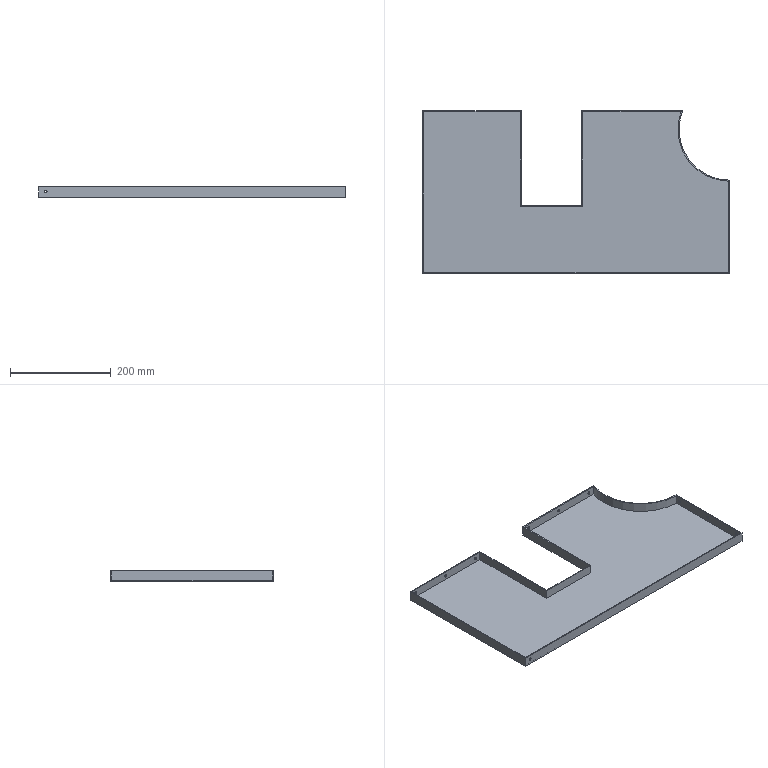Part | SolidWorks | features ICE 3, Extrusion 1, Shell 1 | 1 solid | 43 faces | box 609 x 323 x 20 mm | volume 403774 mm3 | cylinder 24 | plane 19 | commonest cylinder face diameters 5.5 x20 200 x2 204 x2
STEP:
#1=CARTESIAN_POINT('',(609.,174.,8.25));
#2=VERTEX_POINT('',#1);
#3=CARTESIAN_POINT('',(609.,174.,13.75));
#4=VERTEX_POINT('',#3);
#5=CARTESIAN_POINT('',(609.,174.,11.));
#6=DIRECTION('',(-1.,0.,0.));
#7=DIRECTION('',(0.,0.,1.));
#8=AXIS2_PLACEMENT_3D('',#5,#6,#7);
#9=CIRCLE('',#8,2.75);
#10=EDGE_CURVE('',#2,#4,#9,.T.);
#11=ORIENTED_EDGE('',*,*,#10,.F.);
#12=CARTESIAN_POINT('',(607.,174.,8.25));
#13=VERTEX_POINT('',#12);
#14=CARTESIAN_POINT('',(617.,174.,8.25));
#15=DIRECTION('',(-1.,0.,0.));
#16=VECTOR('',#15,1000.);
#17=LINE('',#14,#16);
#18=EDGE_CURVE('',#2,#13,#17,.T.);
#19=ORIENTED_EDGE('',*,*,#18,.T.);
#20=CARTESIAN_POINT('',(607.,174.,13.75));
#21=VERTEX_POINT('',#20);
#22=CARTESIAN_POINT('',(607.,174.,11.));
#23=DIRECTION('',(-1.,0.,0.));
#24=DIRECTION('',(0.,0.,1.));
#25=AXIS2_PLACEMENT_3D('',#22,#23,#24);
#26=CIRCLE('',#25,2.75);
#27=EDGE_CURVE('',#13,#21,#26,.T.);
#28=ORIENTED_EDGE('',*,*,#27,.T.);
#29=CARTESIAN_POINT('',(617.,174.,13.75));
#30=DIRECTION('',(-1.,0.,0.));
#31=VECTOR('',#30,1000.);
#32=LINE('',#29,#31);
#33=EDGE_CURVE('',#4,#21,#32,.T.);
#34=ORIENTED_EDGE('',*,*,#33,.F.);
#35=EDGE_LOOP('',(#11,#19,#28,#34));
#36=FACE_OUTER_BOUND('',#35,.T.);
#37=CARTESIAN_POINT('',(617.,174.,11.));
#38=DIRECTION('',(-1.,0.,0.));
#39=DIRECTION('',(0.,0.,1.));
#40=AXIS2_PLACEMENT_3D('',#37,#38,#39);
#41=CYLINDRICAL_SURFACE('',#40,2.75);
#42=ADVANCED_FACE('',(#36),#41,.F.);
#43=CARTESIAN_POINT('',(609.,94.,8.25));
#44=VERTEX_POINT('',#43);
#45=CARTESIAN_POINT('',(609.,94.,13.75));
#46=VERTEX_POINT('',#45);
#47=CARTESIAN_POINT('',(609.,94.,11.));
#48=DIRECTION('',(-1.,0.,0.));
#49=DIRECTION('',(0.,0.,1.));
#50=AXIS2_PLACEMENT_3D('',#47,#48,#49);
#51=CIRCLE('',#50,2.75);
#52=EDGE_CURVE('',#44,#46,#51,.T.);
#53=ORIENTED_EDGE('',*,*,#52,.F.);
#54=CARTESIAN_POINT('',(607.,94.,8.25));
#55=VERTEX_POINT('',#54);
#56=CARTESIAN_POINT('',(617.,94.,8.25));
#57=DIRECTION('',(-1.,0.,0.));
#58=VECTOR('',#57,1000.);
#59=LINE('',#56,#58);
#60=EDGE_CURVE('',#44,#55,#59,.T.);
#61=ORIENTED_EDGE('',*,*,#60,.T.);
#62=CARTESIAN_POINT('',(607.,94.,13.75));
#63=VERTEX_POINT('',#62);
#64=CARTESIAN_POINT('',(607.,94.,11.));
#65=DIRECTION('',(-1.,0.,0.));
#66=DIRECTION('',(0.,0.,1.));
#67=AXIS2_PLACEMENT_3D('',#64,#65,#66);
#68=CIRCLE('',#67,2.75);
#69=EDGE_CURVE('',#55,#63,#68,.T.);
#70=ORIENTED_EDGE('',*,*,#69,.T.);
#71=CARTESIAN_POINT('',(617.,94.,13.75));
#72=DIRECTION('',(-1.,0.,0.));
#73=VECTOR('',#72,1000.);
#74=LINE('',#71,#73);
#75=EDGE_CURVE('',#46,#63,#74,.T.);
#76=ORIENTED_EDGE('',*,*,#75,.F.);
#77=EDGE_LOOP('',(#53,#61,#70,#76));
#78=FACE_OUTER_BOUND('',#77,.T.);
#79=CARTESIAN_POINT('',(617.,94.,11.));
#80=DIRECTION('',(-1.,0.,0.));
#81=DIRECTION('',(0.,0.,1.));
#82=AXIS2_PLACEMENT_3D('',#79,#80,#81);
#83=CYLINDRICAL_SURFACE('',#82,2.75);
#84=ADVANCED_FACE('',(#78),#83,.F.);
#85=CARTESIAN_POINT('',(609.,14.,8.25));
#86=VERTEX_POINT('',#85);
#87=CARTESIAN_POINT('',(609.,14.,13.75));
#88=VERTEX_POINT('',#87);
#89=CARTESIAN_POINT('',(609.,14.,11.));
#90=DIRECTION('',(-1.,0.,0.));
#91=DIRECTION('',(0.,0.,1.));
#92=AXIS2_PLACEMENT_3D('',#89,#90,#91);
#93=CIRCLE('',#92,2.75);
#94=EDGE_CURVE('',#86,#88,#93,.T.);
#95=ORIENTED_EDGE('',*,*,#94,.F.);
#96=CARTESIAN_POINT('',(607.,14.,8.25));
#97=VERTEX_POINT('',#96);
#98=CARTESIAN_POINT('',(617.,14.,8.25));
#99=DIRECTION('',(-1.,0.,0.));
#100=VECTOR('',#99,1000.);
#101=LINE('',#98,#100);
#102=EDGE_CURVE('',#86,#97,#101,.T.);
#103=ORIENTED_EDGE('',*,*,#102,.T.);
#104=CARTESIAN_POINT('',(607.,14.,13.75));
#105=VERTEX_POINT('',#104);
#106=CARTESIAN_POINT('',(607.,14.,11.));
#107=DIRECTION('',(-1.,0.,0.));
#108=DIRECTION('',(0.,0.,1.));
#109=AXIS2_PLACEMENT_3D('',#106,#107,#108);
#110=CIRCLE('',#109,2.75);
#111=EDGE_CURVE('',#97,#105,#110,.T.);
#112=ORIENTED_EDGE('',*,*,#111,.T.);
#113=CARTESIAN_POINT('',(617.,14.,13.75));
#114=DIRECTION('',(-1.,0.,0.));
#115=VECTOR('',#114,1000.);
#116=LINE('',#113,#115);
#117=EDGE_CURVE('',#88,#105,#116,.T.);
#118=ORIENTED_EDGE('',*,*,#117,.F.);
#119=EDGE_LOOP('',(#95,#103,#112,#118));
#120=FACE_OUTER_BOUND('',#119,.T.);
#121=CARTESIAN_POINT('',(617.,14.,11.));
#122=DIRECTION('',(-1.,0.,0.));
#123=DIRECTION('',(0.,0.,1.));
#124=AXIS2_PLACEMENT_3D('',#121,#122,#123);
#125=CYLINDRICAL_SURFACE('',#124,2.75);
#126=ADVANCED_FACE('',(#120),#125,.F.);
#127=CARTESIAN_POINT('',(500.,323.,13.75));
#128=VERTEX_POINT('',#127);
#129=CARTESIAN_POINT('',(500.,323.,8.25));
#130=VERTEX_POINT('',#129);
#131=CARTESIAN_POINT('',(500.,323.,11.));
#132=DIRECTION('',(0.,-1.,0.));
#133=DIRECTION('',(1.,0.,0.));
#134=AXIS2_PLACEMENT_3D('',#131,#132,#133);
#135=CIRCLE('',#134,2.75);
#136=EDGE_CURVE('',#128,#130,#135,.T.);
#137=ORIENTED_EDGE('',*,*,#136,.F.);
#138=CARTESIAN_POINT('',(500.,321.,13.75));
#139=VERTEX_POINT('',#138);
#140=CARTESIAN_POINT('',(500.,331.,13.75));
#141=DIRECTION('',(0.,-1.,0.));
#142=VECTOR('',#141,1000.);
#143=LINE('',#140,#142);
#144=EDGE_CURVE('',#128,#139,#143,.T.);
#145=ORIENTED_EDGE('',*,*,#144,.T.);
#146=CARTESIAN_POINT('',(500.,321.,8.25));
#147=VERTEX_POINT('',#146);
#148=CARTESIAN_POINT('',(500.,321.,11.));
#149=DIRECTION('',(0.,-1.,0.));
#150=DIRECTION('',(0.,0.,-1.));
#151=AXIS2_PLACEMENT_3D('',#148,#149,#150);
#152=CIRCLE('',#151,2.75);
#153=EDGE_CURVE('',#139,#147,#152,.T.);
#154=ORIENTED_EDGE('',*,*,#153,.T.);
#155=CARTESIAN_POINT('',(500.,331.,8.25));
#156=DIRECTION('',(0.,-1.,0.));
#157=VECTOR('',#156,1000.);
#158=LINE('',#155,#157);
#159=EDGE_CURVE('',#130,#147,#158,.T.);
#160=ORIENTED_EDGE('',*,*,#159,.F.);
#161=EDGE_LOOP('',(#137,#145,#154,#160));
#162=FACE_OUTER_BOUND('',#161,.T.);
#163=CARTESIAN_POINT('',(500.,331.,11.));
#164=DIRECTION('',(0.,-1.,0.));
#165=DIRECTION('',(0.,0.,-1.));
#166=AXIS2_PLACEMENT_3D('',#163,#164,#165);
#167=CYLINDRICAL_SURFACE('',#166,2.75);
#168=ADVANCED_FACE('',(#162),#167,.F.);
#169=CARTESIAN_POINT('',(415.,323.,13.75));
#170=VERTEX_POINT('',#169);
#171=CARTESIAN_POINT('',(415.,323.,8.25));
#172=VERTEX_POINT('',#171);
#173=CARTESIAN_POINT('',(415.,323.,11.));
#174=DIRECTION('',(0.,-1.,0.));
#175=DIRECTION('',(1.,0.,0.));
#176=AXIS2_PLACEMENT_3D('',#173,#174,#175);
#177=CIRCLE('',#176,2.75);
#178=EDGE_CURVE('',#170,#172,#177,.T.);
#179=ORIENTED_EDGE('',*,*,#178,.F.);
#180=CARTESIAN_POINT('',(415.,321.,13.75));
#181=VERTEX_POINT('',#180);
#182=CARTESIAN_POINT('',(415.,331.,13.75));
#183=DIRECTION('',(0.,-1.,0.));
#184=VECTOR('',#183,1000.);
#185=LINE('',#182,#184);
#186=EDGE_CURVE('',#170,#181,#185,.T.);
#187=ORIENTED_EDGE('',*,*,#186,.T.);
#188=CARTESIAN_POINT('',(415.,321.,8.25));
#189=VERTEX_POINT('',#188);
#190=CARTESIAN_POINT('',(415.,321.,11.));
#191=DIRECTION('',(0.,-1.,0.));
#192=DIRECTION('',(0.,0.,-1.));
#193=AXIS2_PLACEMENT_3D('',#190,#191,#192);
#194=CIRCLE('',#193,2.75);
#195=EDGE_CURVE('',#181,#189,#194,.T.);
#196=ORIENTED_EDGE('',*,*,#195,.T.);
#197=CARTESIAN_POINT('',(415.,331.,8.25));
#198=DIRECTION('',(0.,-1.,0.));
#199=VECTOR('',#198,1000.);
#200=LINE('',#197,#199);
#201=EDGE_CURVE('',#172,#189,#200,.T.);
#202=ORIENTED_EDGE('',*,*,#201,.F.);
#203=EDGE_LOOP('',(#179,#187,#196,#202));
#204=FACE_OUTER_BOUND('',#203,.T.);
#205=CARTESIAN_POINT('',(415.,331.,11.));
#206=DIRECTION('',(0.,-1.,0.));
#207=DIRECTION('',(0.,0.,-1.));
#208=AXIS2_PLACEMENT_3D('',#205,#206,#207);
#209=CYLINDRICAL_SURFACE('',#208,2.75);
#210=ADVANCED_FACE('',(#204),#209,.F.);
#211=CARTESIAN_POINT('',(330.,323.,13.75));
#212=VERTEX_POINT('',#211);
#213=CARTESIAN_POINT('',(330.,323.,8.25));
#214=VERTEX_POINT('',#213);
#215=CARTESIAN_POINT('',(330.,323.,11.));
#216=DIRECTION('',(0.,-1.,0.));
#217=DIRECTION('',(1.,0.,0.));
#218=AXIS2_PLACEMENT_3D('',#215,#216,#217);
#219=CIRCLE('',#218,2.75);
#220=EDGE_CURVE('',#212,#214,#219,.T.);
#221=ORIENTED_EDGE('',*,*,#220,.F.);
#222=CARTESIAN_POINT('',(330.,321.,13.75));
#223=VERTEX_POINT('',#222);
#224=CARTESIAN_POINT('',(330.,331.,13.75));
#225=DIRECTION('',(0.,-1.,0.));
#226=VECTOR('',#225,1000.);
#227=LINE('',#224,#226);
#228=EDGE_CURVE('',#212,#223,#227,.T.);
#229=ORIENTED_EDGE('',*,*,#228,.T.);
#230=CARTESIAN_POINT('',(330.,321.,8.25));
#231=VERTEX_POINT('',#230);
#232=CARTESIAN_POINT('',(330.,321.,11.));
#233=DIRECTION('',(0.,-1.,0.));
#234=DIRECTION('',(0.,0.,-1.));
#235=AXIS2_PLACEMENT_3D('',#232,#233,#234);
#236=CIRCLE('',#235,2.75);
#237=EDGE_CURVE('',#223,#231,#236,.T.);
#238=ORIENTED_EDGE('',*,*,#237,.T.);
#239=CARTESIAN_POINT('',(330.,331.,8.25));
#240=DIRECTION('',(0.,-1.,0.));
#241=VECTOR('',#240,1000.);
#242=LINE('',#239,#241);
#243=EDGE_CURVE('',#214,#231,#242,.T.);
#244=ORIENTED_EDGE('',*,*,#243,.F.);
#245=EDGE_LOOP('',(#221,#229,#238,#244));
#246=FACE_OUTER_BOUND('',#245,.T.);
#247=CARTESIAN_POINT('',(330.,331.,11.));
#248=DIRECTION('',(0.,-1.,0.));
#249=DIRECTION('',(0.,0.,-1.));
#250=AXIS2_PLACEMENT_3D('',#247,#248,#249);
#251=CYLINDRICAL_SURFACE('',#250,2.75);
#252=ADVANCED_FACE('',(#246),#251,.F.);
#253=CARTESIAN_POINT('',(182.,323.,13.75));
#254=VERTEX_POINT('',#253);
#255=CARTESIAN_POINT('',(182.,323.,8.25));
#256=VERTEX_POINT('',#255);
#257=CARTESIAN_POINT('',(182.,323.,11.));
#258=DIRECTION('',(0.,-1.,0.));
#259=DIRECTION('',(0.,0.,-1.));
#260=AXIS2_PLACEMENT_3D('',#257,#258,#259);
#261=CIRCLE('',#260,2.75);
#262=EDGE_CURVE('',#254,#256,#261,.T.);
#263=ORIENTED_EDGE('',*,*,#262,.F.);
#264=CARTESIAN_POINT('',(182.,321.,13.75));
#265=VERTEX_POINT('',#264);
#266=CARTESIAN_POINT('',(182.,331.,13.75));
#267=DIRECTION('',(0.,-1.,0.));
#268=VECTOR('',#267,1000.);
#269=LINE('',#266,#268);
#270=EDGE_CURVE('',#254,#265,#269,.T.);
#271=ORIENTED_EDGE('',*,*,#270,.T.);
#272=CARTESIAN_POINT('',(182.,321.,8.25));
#273=VERTEX_POINT('',#272);
#274=CARTESIAN_POINT('',(182.,321.,11.));
#275=DIRECTION('',(0.,-1.,0.));
#276=DIRECTION('',(0.,0.,-1.));
#277=AXIS2_PLACEMENT_3D('',#274,#275,#276);
#278=CIRCLE('',#277,2.75);
#279=EDGE_CURVE('',#265,#273,#278,.T.);
#280=ORIENTED_EDGE('',*,*,#279,.T.);
#281=CARTESIAN_POINT('',(182.,331.,8.25));
#282=DIRECTION('',(0.,-1.,0.));
#283=VECTOR('',#282,1000.);
#284=LINE('',#281,#283);
#285=EDGE_CURVE('',#256,#273,#284,.T.);
#286=ORIENTED_EDGE('',*,*,#285,.F.);
#287=EDGE_LOOP('',(#263,#271,#280,#286));
#288=FACE_OUTER_BOUND('',#287,.T.);
#289=CARTESIAN_POINT('',(182.,331.,11.));
#290=DIRECTION('',(0.,-1.,0.));
#291=DIRECTION('',(0.,0.,-1.));
#292=AXIS2_PLACEMENT_3D('',#289,#290,#291);
#293=CYLINDRICAL_SURFACE('',#292,2.75);
#294=ADVANCED_FACE('',(#288),#293,.F.);
#295=CARTESIAN_POINT('',(98.,323.,13.75));
#296=VERTEX_POINT('',#295);
#297=CARTESIAN_POINT('',(98.,323.,8.25));
#298=VERTEX_POINT('',#297);
#299=CARTESIAN_POINT('',(98.,323.,11.));
#300=DIRECTION('',(0.,-1.,0.));
#301=DIRECTION('',(0.,0.,-1.));
#302=AXIS2_PLACEMENT_3D('',#299,#300,#301);
#303=CIRCLE('',#302,2.75);
#304=EDGE_CURVE('',#296,#298,#303,.T.);
#305=ORIENTED_EDGE('',*,*,#304,.F.);
#306=CARTESIAN_POINT('',(98.,321.,13.75));
#307=VERTEX_POINT('',#306);
#308=CARTESIAN_POINT('',(98.,331.,13.75));
#309=DIRECTION('',(0.,-1.,0.));
#310=VECTOR('',#309,1000.);
#311=LINE('',#308,#310);
#312=EDGE_CURVE('',#296,#307,#311,.T.);
#313=ORIENTED_EDGE('',*,*,#312,.T.);
#314=CARTESIAN_POINT('',(98.,321.,8.25));
#315=VERTEX_POINT('',#314);
#316=CARTESIAN_POINT('',(98.,321.,11.));
#317=DIRECTION('',(0.,-1.,0.));
#318=DIRECTION('',(0.,0.,-1.));
#319=AXIS2_PLACEMENT_3D('',#316,#317,#318);
#320=CIRCLE('',#319,2.75);
#321=EDGE_CURVE('',#307,#315,#320,.T.);
#322=ORIENTED_EDGE('',*,*,#321,.T.);
#323=CARTESIAN_POINT('',(98.,331.,8.25));
#324=DIRECTION('',(0.,-1.,0.));
#325=VECTOR('',#324,1000.);
#326=LINE('',#323,#325);
#327=EDGE_CURVE('',#298,#315,#326,.T.);
#328=ORIENTED_EDGE('',*,*,#327,.F.);
#329=EDGE_LOOP('',(#305,#313,#322,#328));
#330=FACE_OUTER_BOUND('',#329,.T.);
#331=CARTESIAN_POINT('',(98.,331.,11.));
#332=DIRECTION('',(0.,-1.,0.));
#333=DIRECTION('',(0.,0.,-1.));
#334=AXIS2_PLACEMENT_3D('',#331,#332,#333);
#335=CYLINDRICAL_SURFACE('',#334,2.75);
#336=ADVANCED_FACE('',(#330),#335,.F.);
#337=CARTESIAN_POINT('',(14.,2.,13.75));
#338=VERTEX_POINT('',#337);
#339=CARTESIAN_POINT('',(14.,2.,8.25));
#340=VERTEX_POINT('',#339);
#341=CARTESIAN_POINT('',(14.,2.,11.));
#342=DIRECTION('',(0.,-1.,0.));
#343=DIRECTION('',(0.,0.,1.));
#344=AXIS2_PLACEMENT_3D('',#341,#342,#343);
#345=CIRCLE('',#344,2.75);
#346=EDGE_CURVE('',#338,#340,#345,.T.);
#347=ORIENTED_EDGE('',*,*,#346,.F.);
#348=CARTESIAN_POINT('',(14.,0.,13.75));
#349=VERTEX_POINT('',#348);
#350=CARTESIAN_POINT('',(14.,340.,13.75));
#351=DIRECTION('',(0.,-1.,0.));
#352=VECTOR('',#351,1000.);
#353=LINE('',#350,#352);
#354=EDGE_CURVE('',#338,#349,#353,.T.);
#355=ORIENTED_EDGE('',*,*,#354,.T.);
#356=CARTESIAN_POINT('',(14.,0.,8.25));
#357=VERTEX_POINT('',#356);
#358=CARTESIAN_POINT('',(14.,0.,11.));
#359=DIRECTION('',(0.,-1.,0.));
#360=DIRECTION('',(0.,0.,1.));
#361=AXIS2_PLACEMENT_3D('',#358,#359,#360);
#362=CIRCLE('',#361,2.75);
#363=EDGE_CURVE('',#349,#357,#362,.T.);
#364=ORIENTED_EDGE('',*,*,#363,.T.);
#365=CARTESIAN_POINT('',(14.,340.,8.25));
#366=DIRECTION('',(0.,-1.,0.));
#367=VECTOR('',#366,1000.);
#368=LINE('',#365,#367);
#369=EDGE_CURVE('',#340,#357,#368,.T.);
#370=ORIENTED_EDGE('',*,*,#369,.F.);
#371=EDGE_LOOP('',(#347,#355,#364,#370));
#372=FACE_OUTER_BOUND('',#371,.T.);
#373=CARTESIAN_POINT('',(14.,340.,11.));
#374=DIRECTION('',(0.,-1.,0.));
#375=DIRECTION('',(0.,0.,-1.));
#376=AXIS2_PLACEMENT_3D('',#373,#374,#375);
#377=CYLINDRICAL_SURFACE('',#376,2.75);
#378=ADVANCED_FACE('',(#372),#377,.F.);
#379=CARTESIAN_POINT('',(14.,323.,8.25));
#380=VERTEX_POINT('',#379);
#381=CARTESIAN_POINT('',(14.,323.,13.75));
#382=VERTEX_POINT('',#381);
#383=CARTESIAN_POINT('',(14.,323.,11.));
#384=DIRECTION('',(0.,1.,0.));
#385=DIRECTION('',(0.,0.,-1.));
#386=AXIS2_PLACEMENT_3D('',#383,#384,#385);
#387=CIRCLE('',#386,2.75);
#388=EDGE_CURVE('',#380,#382,#387,.T.);
#389=ORIENTED_EDGE('',*,*,#388,.T.);
#390=CARTESIAN_POINT('',(14.,321.,13.75));
#391=VERTEX_POINT('',#390);
#392=CARTESIAN_POINT('',(14.,340.,13.75));
#393=DIRECTION('',(0.,-1.,0.));
#394=VECTOR('',#393,1000.);
#395=LINE('',#392,#394);
#396=EDGE_CURVE('',#382,#391,#395,.T.);
#397=ORIENTED_EDGE('',*,*,#396,.T.);
#398=CARTESIAN_POINT('',(14.,321.,8.25));
#399=VERTEX_POINT('',#398);
#400=CARTESIAN_POINT('',(14.,321.,11.));
#401=DIRECTION('',(0.,1.,0.));
#402=DIRECTION('',(0.,0.,-1.));
#403=AXIS2_PLACEMENT_3D('',#400,#401,#402);
#404=CIRCLE('',#403,2.75);
#405=EDGE_CURVE('',#399,#391,#404,.T.);
#406=ORIENTED_EDGE('',*,*,#405,.F.);
#407=CARTESIAN_POINT('',(14.,340.,8.25));
#408=DIRECTION('',(0.,-1.,0.));
#409=VECTOR('',#408,1000.);
#410=LINE('',#407,#409);
#411=EDGE_CURVE('',#380,#399,#410,.T.);
#412=ORIENTED_EDGE('',*,*,#411,.F.);
#413=EDGE_LOOP('',(#389,#397,#406,#412));
#414=FACE_OUTER_BOUND('',#413,.T.);
#415=CARTESIAN_POINT('',(14.,340.,11.));
#416=DIRECTION('',(0.,-1.,0.));
#417=DIRECTION('',(0.,0.,-1.));
#418=AXIS2_PLACEMENT_3D('',#415,#416,#417);
#419=CYLINDRICAL_SURFACE('',#418,2.75);
#420=ADVANCED_FACE('',(#414),#419,.F.);
#421=CARTESIAN_POINT('',(607.,183.02,20.));
#422=VERTEX_POINT('',#421);
#423=CARTESIAN_POINT('',(507.,285.,20.));
#424=VERTEX_POINT('',#423);
#425=CARTESIAN_POINT('',(609.,285.,20.));
#426=DIRECTION('',(0.,0.,-1.));
#427=DIRECTION('',(1.,0.,0.));
#428=AXIS2_PLACEMENT_3D('',#425,#426,#427);
#429=CIRCLE('',#428,102.);
#430=EDGE_CURVE('',#422,#424,#429,.T.);
#431=ORIENTED_EDGE('',*,*,#430,.T.);
#432=CARTESIAN_POINT('',(507.,285.,2.));
#433=VERTEX_POINT('',#432);
#434=CARTESIAN_POINT('',(507.,285.,20.));
#435=DIRECTION('',(0.,0.,-1.));
#436=VECTOR('',#435,1000.);
#437=LINE('',#434,#436);
#438=EDGE_CURVE('',#424,#433,#437,.T.);
#439=ORIENTED_EDGE('',*,*,#438,.T.);
#440=CARTESIAN_POINT('',(607.,183.02,2.));
#441=VERTEX_POINT('',#440);
#442=CARTESIAN_POINT('',(609.,285.,2.));
#443=DIRECTION('',(0.,0.,-1.));
#444=DIRECTION('',(1.,0.,0.));
#445=AXIS2_PLACEMENT_3D('',#442,#443,#444);
#446=CIRCLE('',#445,102.);
#447=EDGE_CURVE('',#441,#433,#446,.T.);
#448=ORIENTED_EDGE('',*,*,#447,.F.);
#449=CARTESIAN_POINT('',(607.,183.02,20.));
#450=DIRECTION('',(0.,0.,-1.));
#451=VECTOR('',#450,1000.);
#452=LINE('',#449,#451);
#453=EDGE_CURVE('',#422,#441,#452,.T.);
#454=ORIENTED_EDGE('',*,*,#453,.F.);
#455=EDGE_LOOP('',(#431,#439,#448,#454));
#456=FACE_OUTER_BOUND('',#455,.T.);
#457=CARTESIAN_POINT('',(609.,285.,20.));
#458=DIRECTION('',(0.,0.,-1.));
#459=DIRECTION('',(-1.,0.,0.));
#460=AXIS2_PLACEMENT_3D('',#457,#458,#459);
#461=CYLINDRICAL_SURFACE('',#460,102.);
#462=ADVANCED_FACE('',(#456),#461,.T.);
#463=CARTESIAN_POINT('',(509.,285.,20.));
#464=VERTEX_POINT('',#463);
#465=CARTESIAN_POINT('',(516.501,323.,20.));
#466=VERTEX_POINT('',#465);
#467=CARTESIAN_POINT('',(609.,285.,20.));
#468=DIRECTION('',(0.,0.,-1.));
#469=DIRECTION('',(1.,0.,0.));
#470=AXIS2_PLACEMENT_3D('',#467,#468,#469);
#471=CIRCLE('',#470,100.);
#472=EDGE_CURVE('',#464,#466,#471,.T.);
#473=ORIENTED_EDGE('',*,*,#472,.F.);
#474=CARTESIAN_POINT('',(509.,285.,0.));
#475=VERTEX_POINT('',#474);
#476=CARTESIAN_POINT('',(509.,285.,20.));
#477=DIRECTION('',(0.,0.,-1.));
#478=VECTOR('',#477,1000.);
#479=LINE('',#476,#478);
#480=EDGE_CURVE('',#464,#475,#479,.T.);
#481=ORIENTED_EDGE('',*,*,#480,.T.);
#482=CARTESIAN_POINT('',(516.501,323.,0.));
#483=VERTEX_POINT('',#482);
#484=CARTESIAN_POINT('',(609.,285.,0.));
#485=DIRECTION('',(0.,0.,-1.));
#486=DIRECTION('',(1.,0.,0.));
#487=AXIS2_PLACEMENT_3D('',#484,#485,#486);
#488=CIRCLE('',#487,100.);
#489=EDGE_CURVE('',#475,#483,#488,.T.);
#490=ORIENTED_EDGE('',*,*,#489,.T.);
#491=CARTESIAN_POINT('',(516.501,323.,20.));
#492=DIRECTION('',(0.,0.,-1.));
#493=VECTOR('',#492,1000.);
#494=LINE('',#491,#493);
#495=EDGE_CURVE('',#466,#483,#494,.T.);
#496=ORIENTED_EDGE('',*,*,#495,.F.);
#497=EDGE_LOOP('',(#473,#481,#490,#496));
#498=FACE_OUTER_BOUND('',#497,.T.);
#499=CARTESIAN_POINT('',(609.,285.,20.));
#500=DIRECTION('',(0.,0.,-1.));
#501=DIRECTION('',(-1.,0.,0.));
#502=AXIS2_PLACEMENT_3D('',#499,#500,#501);
#503=CYLINDRICAL_SURFACE('',#502,100.);
#504=ADVANCED_FACE('',(#498),#503,.F.);
#505=CARTESIAN_POINT('',(0.,0.,0.));
#506=VERTEX_POINT('',#505);
#507=CARTESIAN_POINT('',(609.,0.,0.));
#508=VERTEX_POINT('',#507);
#509=CARTESIAN_POINT('',(0.,0.,0.));
#510=DIRECTION('',(1.,0.,0.));
#511=VECTOR('',#510,1000.);
#512=LINE('',#509,#511);
#513=EDGE_CURVE('',#506,#508,#512,.T.);
#514=ORIENTED_EDGE('',*,*,#513,.T.);
#515=CARTESIAN_POINT('',(609.,0.,20.));
#516=VERTEX_POINT('',#515);
#517=CARTESIAN_POINT('',(609.,0.,20.));
#518=DIRECTION('',(0.,0.,-1.));
#519=VECTOR('',#518,1000.);
#520=LINE('',#517,#519);
#521=EDGE_CURVE('',#516,#508,#520,.T.);
#522=ORIENTED_EDGE('',*,*,#521,.F.);
#523=CARTESIAN_POINT('',(0.,0.,20.));
#524=VERTEX_POINT('',#523);
#525=CARTESIAN_POINT('',(0.,0.,20.));
#526=DIRECTION('',(1.,0.,0.));
#527=VECTOR('',#526,1000.);
#528=LINE('',#525,#527);
#529=EDGE_CURVE('',#524,#516,#528,.T.);
#530=ORIENTED_EDGE('',*,*,#529,.F.);
#531=CARTESIAN_POINT('',(0.,0.,20.));
#532=DIRECTION('',(0.,0.,-1.));
#533=VECTOR('',#532,1000.);
#534=LINE('',#531,#533);
#535=EDGE_CURVE('',#524,#506,#534,.T.);
#536=ORIENTED_EDGE('',*,*,#535,.T.);
#537=EDGE_LOOP('',(#514,#522,#530,#536));
#538=FACE_OUTER_BOUND('',#537,.T.);
#539=CARTESIAN_POINT('',(14.,0.,11.));
#540=DIRECTION('',(0.,-1.,0.));
#541=DIRECTION('',(0.,0.,1.));
#542=AXIS2_PLACEMENT_3D('',#539,#540,#541);
#543=CIRCLE('',#542,2.75);
#544=EDGE_CURVE('',#357,#349,#543,.T.);
#545=ORIENTED_EDGE('',*,*,#544,.F.);
#546=ORIENTED_EDGE('',*,*,#363,.F.);
#547=EDGE_LOOP('',(#545,#546));
#548=FACE_BOUND('',#547,.T.);
#549=CARTESIAN_POINT('',(0.,0.,20.));
#550=DIRECTION('',(0.,1.,0.));
#551=DIRECTION('',(0.,0.,1.));
#552=AXIS2_PLACEMENT_3D('',#549,#550,#551);
#553=PLANE('',#552);
#554=ADVANCED_FACE('',(#538,#548),#553,.F.);
#555=CARTESIAN_POINT('',(182.,323.,11.));
#556=DIRECTION('',(0.,-1.,0.));
#557=DIRECTION('',(0.,0.,-1.));
#558=AXIS2_PLACEMENT_3D('',#555,#556,#557);
#559=CIRCLE('',#558,2.75);
#560=EDGE_CURVE('',#256,#254,#559,.T.);
#561=ORIENTED_EDGE('',*,*,#560,.T.);
#562=ORIENTED_EDGE('',*,*,#262,.T.);
#563=EDGE_LOOP('',(#561,#562));
#564=FACE_BOUND('',#563,.T.);
#565=CARTESIAN_POINT('',(98.,323.,11.));
#566=DIRECTION('',(0.,-1.,0.));
#567=DIRECTION('',(0.,0.,-1.));
#568=AXIS2_PLACEMENT_3D('',#565,#566,#567);
#569=CIRCLE('',#568,2.75);
#570=EDGE_CURVE('',#298,#296,#569,.T.);
#571=ORIENTED_EDGE('',*,*,#570,.T.);
#572=ORIENTED_EDGE('',*,*,#304,.T.);
#573=EDGE_LOOP('',(#571,#572));
#574=FACE_BOUND('',#573,.T.);
#575=CARTESIAN_POINT('',(196.,323.,0.));
#576=VERTEX_POINT('',#575);
#577=CARTESIAN_POINT('',(0.,323.,0.));
#578=VERTEX_POINT('',#577);
#579=CARTESIAN_POINT('',(0.,323.,0.));
#580=DIRECTION('',(-1.,0.,0.));
#581=VECTOR('',#580,1000.);
#582=LINE('',#579,#581);
#583=EDGE_CURVE('',#576,#578,#582,.T.);
#584=ORIENTED_EDGE('',*,*,#583,.T.);
#585=CARTESIAN_POINT('',(0.,323.,20.));
#586=VERTEX_POINT('',#585);
#587=CARTESIAN_POINT('',(0.,323.,20.));
#588=DIRECTION('',(0.,0.,-1.));
#589=VECTOR('',#588,1000.);
#590=LINE('',#587,#589);
#591=EDGE_CURVE('',#586,#578,#590,.T.);
#592=ORIENTED_EDGE('',*,*,#591,.F.);
#593=CARTESIAN_POINT('',(196.,323.,20.));
#594=VERTEX_POINT('',#593);
#595=CARTESIAN_POINT('',(0.,323.,20.));
#596=DIRECTION('',(-1.,0.,0.));
#597=VECTOR('',#596,1000.);
#598=LINE('',#595,#597);
#599=EDGE_CURVE('',#594,#586,#598,.T.);
#600=ORIENTED_EDGE('',*,*,#599,.F.);
#601=CARTESIAN_POINT('',(196.,323.,20.));
#602=DIRECTION('',(0.,0.,-1.));
#603=VECTOR('',#602,1000.);
#604=LINE('',#601,#603);
#605=EDGE_CURVE('',#594,#576,#604,.T.);
#606=ORIENTED_EDGE('',*,*,#605,.T.);
#607=EDGE_LOOP('',(#584,#592,#600,#606));
#608=FACE_OUTER_BOUND('',#607,.T.);
#609=ORIENTED_EDGE('',*,*,#388,.F.);
#610=CARTESIAN_POINT('',(14.,323.,11.));
#611=DIRECTION('',(0.,1.,0.));
#612=DIRECTION('',(0.,0.,-1.));
#613=AXIS2_PLACEMENT_3D('',#610,#611,#612);
#614=CIRCLE('',#613,2.75);
#615=EDGE_CURVE('',#382,#380,#614,.T.);
#616=ORIENTED_EDGE('',*,*,#615,.F.);
#617=EDGE_LOOP('',(#609,#616));
#618=FACE_BOUND('',#617,.T.);
#619=CARTESIAN_POINT('',(0.,323.,20.));
#620=DIRECTION('',(0.,-1.,0.));
#621=DIRECTION('',(0.,0.,-1.));
#622=AXIS2_PLACEMENT_3D('',#619,#620,#621);
#623=PLANE('',#622);
#624=ADVANCED_FACE('',(#564,#574,#608,#618),#623,.F.);
#625=CARTESIAN_POINT('',(2.,2.,2.));
#626=VERTEX_POINT('',#625);
#627=CARTESIAN_POINT('',(607.,2.,2.));
#628=VERTEX_POINT('',#627);
#629=CARTESIAN_POINT('',(0.,2.,2.));
#630=DIRECTION('',(1.,0.,0.));
#631=VECTOR('',#630,1000.);
#632=LINE('',#629,#631);
#633=EDGE_CURVE('',#626,#628,#632,.T.);
#634=ORIENTED_EDGE('',*,*,#633,.F.);
#635=CARTESIAN_POINT('',(2.,2.,20.));
#636=VERTEX_POINT('',#635);
#637=CARTESIAN_POINT('',(2.,2.,20.));
#638=DIRECTION('',(0.,0.,-1.));
#639=VECTOR('',#638,1000.);
#640=LINE('',#637,#639);
#641=EDGE_CURVE('',#636,#626,#640,.T.);
#642=ORIENTED_EDGE('',*,*,#641,.F.);
#643=CARTESIAN_POINT('',(607.,2.,20.));
#644=VERTEX_POINT('',#643);
#645=CARTESIAN_POINT('',(0.,2.,20.));
#646=DIRECTION('',(1.,0.,0.));
#647=VECTOR('',#646,1000.);
#648=LINE('',#645,#647);
#649=EDGE_CURVE('',#636,#644,#648,.T.);
#650=ORIENTED_EDGE('',*,*,#649,.T.);
#651=CARTESIAN_POINT('',(607.,2.,20.));
#652=DIRECTION('',(0.,0.,-1.));
#653=VECTOR('',#652,1000.);
#654=LINE('',#651,#653);
#655=EDGE_CURVE('',#644,#628,#654,.T.);
#656=ORIENTED_EDGE('',*,*,#655,.T.);
#657=EDGE_LOOP('',(#634,#642,#650,#656));
#658=FACE_OUTER_BOUND('',#657,.T.);
#659=CARTESIAN_POINT('',(14.,2.,11.));
#660=DIRECTION('',(0.,-1.,0.));
#661=DIRECTION('',(0.,0.,1.));
#662=AXIS2_PLACEMENT_3D('',#659,#660,#661);
#663=CIRCLE('',#662,2.75);
#664=EDGE_CURVE('',#340,#338,#663,.T.);
#665=ORIENTED_EDGE('',*,*,#664,.T.);
#666=ORIENTED_EDGE('',*,*,#346,.T.);
#667=EDGE_LOOP('',(#665,#666));
#668=FACE_BOUND('',#667,.T.);
#669=CARTESIAN_POINT('',(0.,2.,20.));
#670=DIRECTION('',(0.,1.,0.));
#671=DIRECTION('',(0.,0.,1.));
#672=AXIS2_PLACEMENT_3D('',#669,#670,#671);
#673=PLANE('',#672);
#674=ADVANCED_FACE('',(#658,#668),#673,.T.);
#675=CARTESIAN_POINT('',(182.,321.,11.));
#676=DIRECTION('',(0.,-1.,0.));
#677=DIRECTION('',(0.,0.,-1.));
#678=AXIS2_PLACEMENT_3D('',#675,#676,#677);
#679=CIRCLE('',#678,2.75);
#680=EDGE_CURVE('',#273,#265,#679,.T.);
#681=ORIENTED_EDGE('',*,*,#680,.F.);
#682=ORIENTED_EDGE('',*,*,#279,.F.);
#683=EDGE_LOOP('',(#681,#682));
#684=FACE_BOUND('',#683,.T.);
#685=CARTESIAN_POINT('',(98.,321.,11.));
#686=DIRECTION('',(0.,-1.,0.));
#687=DIRECTION('',(0.,0.,-1.));
#688=AXIS2_PLACEMENT_3D('',#685,#686,#687);
#689=CIRCLE('',#688,2.75);
#690=EDGE_CURVE('',#315,#307,#689,.T.);
#691=ORIENTED_EDGE('',*,*,#690,.F.);
#692=ORIENTED_EDGE('',*,*,#321,.F.);
#693=EDGE_LOOP('',(#691,#692));
#694=FACE_BOUND('',#693,.T.);
#695=CARTESIAN_POINT('',(194.,321.,2.));
#696=VERTEX_POINT('',#695);
#697=CARTESIAN_POINT('',(2.,321.,2.));
#698=VERTEX_POINT('',#697);
#699=CARTESIAN_POINT('',(0.,321.,2.));
#700=DIRECTION('',(-1.,0.,0.));
#701=VECTOR('',#700,1000.);
#702=LINE('',#699,#701);
#703=EDGE_CURVE('',#696,#698,#702,.T.);
#704=ORIENTED_EDGE('',*,*,#703,.F.);
#705=CARTESIAN_POINT('',(194.,321.,20.));
#706=VERTEX_POINT('',#705);
#707=CARTESIAN_POINT('',(194.,321.,20.));
#708=DIRECTION('',(0.,0.,-1.));
#709=VECTOR('',#708,1000.);
#710=LINE('',#707,#709);
#711=EDGE_CURVE('',#706,#696,#710,.T.);
#712=ORIENTED_EDGE('',*,*,#711,.F.);
#713=CARTESIAN_POINT('',(2.,321.,20.));
#714=VERTEX_POINT('',#713);
#715=CARTESIAN_POINT('',(0.,321.,20.));
#716=DIRECTION('',(-1.,0.,0.));
#717=VECTOR('',#716,1000.);
#718=LINE('',#715,#717);
#719=EDGE_CURVE('',#706,#714,#718,.T.);
#720=ORIENTED_EDGE('',*,*,#719,.T.);
#721=CARTESIAN_POINT('',(2.,321.,20.));
#722=DIRECTION('',(0.,0.,-1.));
#723=VECTOR('',#722,1000.);
#724=LINE('',#721,#723);
#725=EDGE_CURVE('',#714,#698,#724,.T.);
#726=ORIENTED_EDGE('',*,*,#725,.T.);
#727=EDGE_LOOP('',(#704,#712,#720,#726));
#728=FACE_OUTER_BOUND('',#727,.T.);
#729=ORIENTED_EDGE('',*,*,#405,.T.);
#730=CARTESIAN_POINT('',(14.,321.,11.));
#731=DIRECTION('',(0.,1.,0.));
#732=DIRECTION('',(0.,0.,-1.));
#733=AXIS2_PLACEMENT_3D('',#730,#731,#732);
#734=CIRCLE('',#733,2.75);
#735=EDGE_CURVE('',#391,#399,#734,.T.);
#736=ORIENTED_EDGE('',*,*,#735,.T.);
#737=EDGE_LOOP('',(#729,#736));
#738=FACE_BOUND('',#737,.T.);
#739=CARTESIAN_POINT('',(0.,321.,20.));
#740=DIRECTION('',(0.,-1.,0.));
#741=DIRECTION('',(0.,0.,-1.));
#742=AXIS2_PLACEMENT_3D('',#739,#740,#741);
#743=PLANE('',#742);
#744=ADVANCED_FACE('',(#684,#694,#728,#738),#743,.T.);
#745=CARTESIAN_POINT('',(0.,0.,0.));
#746=DIRECTION('',(0.,-1.,0.));
#747=VECTOR('',#746,1000.);
#748=LINE('',#745,#747);
#749=EDGE_CURVE('',#578,#506,#748,.T.);
#750=ORIENTED_EDGE('',*,*,#749,.T.);
#751=ORIENTED_EDGE('',*,*,#535,.F.);
#752=CARTESIAN_POINT('',(0.,0.,20.));
#753=DIRECTION('',(0.,-1.,0.));
#754=VECTOR('',#753,1000.);
#755=LINE('',#752,#754);
#756=EDGE_CURVE('',#586,#524,#755,.T.);
#757=ORIENTED_EDGE('',*,*,#756,.F.);
#758=ORIENTED_EDGE('',*,*,#591,.T.);
#759=EDGE_LOOP('',(#750,#751,#757,#758));
#760=FACE_OUTER_BOUND('',#759,.T.);
#761=CARTESIAN_POINT('',(0.,0.,20.));
#762=DIRECTION('',(1.,0.,0.));
#763=DIRECTION('',(0.,0.,-1.));
#764=AXIS2_PLACEMENT_3D('',#761,#762,#763);
#765=PLANE('',#764);
#766=ADVANCED_FACE('',(#760),#765,.F.);
#767=CARTESIAN_POINT('',(609.,174.,11.));
#768=DIRECTION('',(-1.,0.,0.));
#769=DIRECTION('',(0.,0.,1.));
#770=AXIS2_PLACEMENT_3D('',#767,#768,#769);
#771=CIRCLE('',#770,2.75);
#772=EDGE_CURVE('',#4,#2,#771,.T.);
#773=ORIENTED_EDGE('',*,*,#772,.T.);
#774=ORIENTED_EDGE('',*,*,#10,.T.);
#775=EDGE_LOOP('',(#773,#774));
#776=FACE_BOUND('',#775,.T.);
#777=CARTESIAN_POINT('',(609.,94.,11.));
#778=DIRECTION('',(-1.,0.,0.));
#779=DIRECTION('',(0.,0.,1.));
#780=AXIS2_PLACEMENT_3D('',#777,#778,#779);
#781=CIRCLE('',#780,2.75);
#782=EDGE_CURVE('',#46,#44,#781,.T.);
#783=ORIENTED_EDGE('',*,*,#782,.T.);
#784=ORIENTED_EDGE('',*,*,#52,.T.);
#785=EDGE_LOOP('',(#783,#784));
#786=FACE_BOUND('',#785,.T.);
#787=CARTESIAN_POINT('',(609.,14.,11.));
#788=DIRECTION('',(-1.,0.,0.));
#789=DIRECTION('',(0.,0.,1.));
#790=AXIS2_PLACEMENT_3D('',#787,#788,#789);
#791=CIRCLE('',#790,2.75);
#792=EDGE_CURVE('',#88,#86,#791,.T.);
#793=ORIENTED_EDGE('',*,*,#792,.T.);
#794=ORIENTED_EDGE('',*,*,#94,.T.);
#795=EDGE_LOOP('',(#793,#794));
#796=FACE_BOUND('',#795,.T.);
#797=CARTESIAN_POINT('',(609.,185.,0.));
#798=VERTEX_POINT('',#797);
#799=CARTESIAN_POINT('',(609.,0.,0.));
#800=DIRECTION('',(0.,1.,0.));
#801=VECTOR('',#800,1000.);
#802=LINE('',#799,#801);
#803=EDGE_CURVE('',#508,#798,#802,.T.);
#804=ORIENTED_EDGE('',*,*,#803,.T.);
#805=CARTESIAN_POINT('',(609.,185.,20.));
#806=VERTEX_POINT('',#805);
#807=CARTESIAN_POINT('',(609.,185.,20.));
#808=DIRECTION('',(0.,0.,-1.));
#809=VECTOR('',#808,1000.);
#810=LINE('',#807,#809);
#811=EDGE_CURVE('',#806,#798,#810,.T.);
#812=ORIENTED_EDGE('',*,*,#811,.F.);
#813=CARTESIAN_POINT('',(609.,0.,20.));
#814=DIRECTION('',(0.,1.,0.));
#815=VECTOR('',#814,1000.);
#816=LINE('',#813,#815);
#817=EDGE_CURVE('',#516,#806,#816,.T.);
#818=ORIENTED_EDGE('',*,*,#817,.F.);
#819=ORIENTED_EDGE('',*,*,#521,.T.);
#820=EDGE_LOOP('',(#804,#812,#818,#819));
#821=FACE_OUTER_BOUND('',#820,.T.);
#822=CARTESIAN_POINT('',(609.,0.,20.));
#823=DIRECTION('',(-1.,0.,0.));
#824=DIRECTION('',(0.,0.,1.));
#825=AXIS2_PLACEMENT_3D('',#822,#823,#824);
#826=PLANE('',#825);
#827=ADVANCED_FACE('',(#776,#786,#796,#821),#826,.F.);
#828=ORIENTED_EDGE('',*,*,#480,.F.);
#829=CARTESIAN_POINT('',(609.,285.,20.));
#830=DIRECTION('',(0.,0.,-1.));
#831=DIRECTION('',(1.,0.,0.));
#832=AXIS2_PLACEMENT_3D('',#829,#830,#831);
#833=CIRCLE('',#832,100.);
#834=EDGE_CURVE('',#806,#464,#833,.T.);
#835=ORIENTED_EDGE('',*,*,#834,.F.);
#836=ORIENTED_EDGE('',*,*,#811,.T.);
#837=CARTESIAN_POINT('',(609.,285.,0.));
#838=DIRECTION('',(0.,0.,-1.));
#839=DIRECTION('',(1.,0.,0.));
#840=AXIS2_PLACEMENT_3D('',#837,#838,#839);
#841=CIRCLE('',#840,100.);
#842=EDGE_CURVE('',#798,#475,#841,.T.);
#843=ORIENTED_EDGE('',*,*,#842,.T.);
#844=EDGE_LOOP('',(#828,#835,#836,#843));
#845=FACE_OUTER_BOUND('',#844,.T.);
#846=CARTESIAN_POINT('',(609.,285.,20.));
#847=DIRECTION('',(0.,0.,-1.));
#848=DIRECTION('',(-1.,0.,0.));
#849=AXIS2_PLACEMENT_3D('',#846,#847,#848);
#850=CYLINDRICAL_SURFACE('',#849,100.);
#851=ADVANCED_FACE('',(#845),#850,.F.);
#852=CARTESIAN_POINT('',(500.,323.,11.));
#853=DIRECTION('',(0.,-1.,0.));
#854=DIRECTION('',(1.,0.,0.));
#855=AXIS2_PLACEMENT_3D('',#852,#853,#854);
#856=CIRCLE('',#855,2.75);
#857=EDGE_CURVE('',#130,#128,#856,.T.);
#858=ORIENTED_EDGE('',*,*,#857,.T.);
#859=ORIENTED_EDGE('',*,*,#136,.T.);
#860=EDGE_LOOP('',(#858,#859));
#861=FACE_BOUND('',#860,.T.);
#862=CARTESIAN_POINT('',(415.,323.,11.));
#863=DIRECTION('',(0.,-1.,0.));
#864=DIRECTION('',(1.,0.,0.));
#865=AXIS2_PLACEMENT_3D('',#862,#863,#864);
#866=CIRCLE('',#865,2.75);
#867=EDGE_CURVE('',#172,#170,#866,.T.);
#868=ORIENTED_EDGE('',*,*,#867,.T.);
#869=ORIENTED_EDGE('',*,*,#178,.T.);
#870=EDGE_LOOP('',(#868,#869));
#871=FACE_BOUND('',#870,.T.);
#872=CARTESIAN_POINT('',(330.,323.,11.));
#873=DIRECTION('',(0.,-1.,0.));
#874=DIRECTION('',(1.,0.,0.));
#875=AXIS2_PLACEMENT_3D('',#872,#873,#874);
#876=CIRCLE('',#875,2.75);
#877=EDGE_CURVE('',#214,#212,#876,.T.);
#878=ORIENTED_EDGE('',*,*,#877,.T.);
#879=ORIENTED_EDGE('',*,*,#220,.T.);
#880=EDGE_LOOP('',(#878,#879));
#881=FACE_BOUND('',#880,.T.);
#882=CARTESIAN_POINT('',(316.,323.,0.));
#883=VERTEX_POINT('',#882);
#884=CARTESIAN_POINT('',(316.,323.,0.));
#885=DIRECTION('',(-1.,0.,0.));
#886=VECTOR('',#885,1000.);
#887=LINE('',#884,#886);
#888=EDGE_CURVE('',#483,#883,#887,.T.);
#889=ORIENTED_EDGE('',*,*,#888,.T.);
#890=CARTESIAN_POINT('',(316.,323.,20.));
#891=VERTEX_POINT('',#890);
#892=CARTESIAN_POINT('',(316.,323.,20.));
#893=DIRECTION('',(0.,0.,-1.));
#894=VECTOR('',#893,1000.);
#895=LINE('',#892,#894);
#896=EDGE_CURVE('',#891,#883,#895,.T.);
#897=ORIENTED_EDGE('',*,*,#896,.F.);
#898=CARTESIAN_POINT('',(316.,323.,20.));
#899=DIRECTION('',(-1.,0.,0.));
#900=VECTOR('',#899,1000.);
#901=LINE('',#898,#900);
#902=EDGE_CURVE('',#466,#891,#901,.T.);
#903=ORIENTED_EDGE('',*,*,#902,.F.);
#904=ORIENTED_EDGE('',*,*,#495,.T.);
#905=EDGE_LOOP('',(#889,#897,#903,#904));
#906=FACE_OUTER_BOUND('',#905,.T.);
#907=CARTESIAN_POINT('',(316.,323.,20.));
#908=DIRECTION('',(0.,-1.,0.));
#909=DIRECTION('',(1.,0.,0.));
#910=AXIS2_PLACEMENT_3D('',#907,#908,#909);
#911=PLANE('',#910);
#912=ADVANCED_FACE('',(#861,#871,#881,#906),#911,.F.);
#913=CARTESIAN_POINT('',(316.,135.,0.));
#914=VERTEX_POINT('',#913);
#915=CARTESIAN_POINT('',(316.,323.,0.));
#916=DIRECTION('',(0.,-1.,0.));
#917=VECTOR('',#916,1000.);
#918=LINE('',#915,#917);
#919=EDGE_CURVE('',#883,#914,#918,.T.);
#920=ORIENTED_EDGE('',*,*,#919,.T.);
#921=CARTESIAN_POINT('',(316.,135.,20.));
#922=VERTEX_POINT('',#921);
#923=CARTESIAN_POINT('',(316.,135.,20.));
#924=DIRECTION('',(0.,0.,-1.));
#925=VECTOR('',#924,1000.);
#926=LINE('',#923,#925);
#927=EDGE_CURVE('',#922,#914,#926,.T.);
#928=ORIENTED_EDGE('',*,*,#927,.F.);
#929=CARTESIAN_POINT('',(316.,323.,20.));
#930=DIRECTION('',(0.,-1.,0.));
#931=VECTOR('',#930,1000.);
#932=LINE('',#929,#931);
#933=EDGE_CURVE('',#891,#922,#932,.T.);
#934=ORIENTED_EDGE('',*,*,#933,.F.);
#935=ORIENTED_EDGE('',*,*,#896,.T.);
#936=EDGE_LOOP('',(#920,#928,#934,#935));
#937=FACE_OUTER_BOUND('',#936,.T.);
#938=CARTESIAN_POINT('',(316.,323.,20.));
#939=DIRECTION('',(1.,0.,0.));
#940=DIRECTION('',(0.,1.,0.));
#941=AXIS2_PLACEMENT_3D('',#938,#939,#940);
#942=PLANE('',#941);
#943=ADVANCED_FACE('',(#937),#942,.F.);
#944=CARTESIAN_POINT('',(196.,135.,0.));
#945=VERTEX_POINT('',#944);
#946=CARTESIAN_POINT('',(196.,135.,0.));
#947=DIRECTION('',(-1.,0.,0.));
#948=VECTOR('',#947,1000.);
#949=LINE('',#946,#948);
#950=EDGE_CURVE('',#914,#945,#949,.T.);
#951=ORIENTED_EDGE('',*,*,#950,.T.);
#952=CARTESIAN_POINT('',(196.,135.,20.));
#953=VERTEX_POINT('',#952);
#954=CARTESIAN_POINT('',(196.,135.,20.));
#955=DIRECTION('',(0.,0.,-1.));
#956=VECTOR('',#955,1000.);
#957=LINE('',#954,#956);
#958=EDGE_CURVE('',#953,#945,#957,.T.);
#959=ORIENTED_EDGE('',*,*,#958,.F.);
#960=CARTESIAN_POINT('',(196.,135.,20.));
#961=DIRECTION('',(-1.,0.,0.));
#962=VECTOR('',#961,1000.);
#963=LINE('',#960,#962);
#964=EDGE_CURVE('',#922,#953,#963,.T.);
#965=ORIENTED_EDGE('',*,*,#964,.F.);
#966=ORIENTED_EDGE('',*,*,#927,.T.);
#967=EDGE_LOOP('',(#951,#959,#965,#966));
#968=FACE_OUTER_BOUND('',#967,.T.);
#969=CARTESIAN_POINT('',(196.,135.,20.));
#970=DIRECTION('',(0.,-1.,0.));
#971=DIRECTION('',(0.,0.,-1.));
#972=AXIS2_PLACEMENT_3D('',#969,#970,#971);
#973=PLANE('',#972);
#974=ADVANCED_FACE('',(#968),#973,.F.);
#975=CARTESIAN_POINT('',(196.,323.,0.));
#976=DIRECTION('',(0.,1.,0.));
#977=VECTOR('',#976,1000.);
#978=LINE('',#975,#977);
#979=EDGE_CURVE('',#945,#576,#978,.T.);
#980=ORIENTED_EDGE('',*,*,#979,.T.);
#981=ORIENTED_EDGE('',*,*,#605,.F.);
#982=CARTESIAN_POINT('',(196.,323.,20.));
#983=DIRECTION('',(0.,1.,0.));
#984=VECTOR('',#983,1000.);
#985=LINE('',#982,#984);
#986=EDGE_CURVE('',#953,#594,#985,.T.);
#987=ORIENTED_EDGE('',*,*,#986,.F.);
#988=ORIENTED_EDGE('',*,*,#958,.T.);
#989=EDGE_LOOP('',(#980,#981,#987,#988));
#990=FACE_OUTER_BOUND('',#989,.T.);
#991=CARTESIAN_POINT('',(196.,323.,20.));
#992=DIRECTION('',(-1.,0.,0.));
#993=DIRECTION('',(0.,-1.,0.));
#994=AXIS2_PLACEMENT_3D('',#991,#992,#993);
#995=PLANE('',#994);
#996=ADVANCED_FACE('',(#990),#995,.F.);
#997=CARTESIAN_POINT('',(2.,0.,20.));
#998=DIRECTION('',(0.,-1.,0.));
#999=VECTOR('',#998,1000.);
#1000=LINE('',#997,#999);
#1001=EDGE_CURVE('',#714,#636,#1000,.T.);
#1002=ORIENTED_EDGE('',*,*,#1001,.F.);
#1003=ORIENTED_EDGE('',*,*,#719,.F.);
#1004=CARTESIAN_POINT('',(194.,133.,20.));
#1005=VERTEX_POINT('',#1004);
#1006=CARTESIAN_POINT('',(194.,323.,20.));
#1007=DIRECTION('',(0.,1.,0.));
#1008=VECTOR('',#1007,1000.);
#1009=LINE('',#1006,#1008);
#1010=EDGE_CURVE('',#1005,#706,#1009,.T.);
#1011=ORIENTED_EDGE('',*,*,#1010,.F.);
#1012=CARTESIAN_POINT('',(318.,133.,20.));
#1013=VERTEX_POINT('',#1012);
#1014=CARTESIAN_POINT('',(196.,133.,20.));
#1015=DIRECTION('',(-1.,0.,0.));
#1016=VECTOR('',#1015,1000.);
#1017=LINE('',#1014,#1016);
#1018=EDGE_CURVE('',#1013,#1005,#1017,.T.);
#1019=ORIENTED_EDGE('',*,*,#1018,.F.);
#1020=CARTESIAN_POINT('',(318.,321.,20.));
#1021=VERTEX_POINT('',#1020);
#1022=CARTESIAN_POINT('',(318.,323.,20.));
#1023=DIRECTION('',(0.,-1.,0.));
#1024=VECTOR('',#1023,1000.);
#1025=LINE('',#1022,#1024);
#1026=EDGE_CURVE('',#1021,#1013,#1025,.T.);
#1027=ORIENTED_EDGE('',*,*,#1026,.F.);
#1028=CARTESIAN_POINT('',(513.564,321.,20.));
#1029=VERTEX_POINT('',#1028);
#1030=CARTESIAN_POINT('',(316.,321.,20.));
#1031=DIRECTION('',(-1.,0.,0.));
#1032=VECTOR('',#1031,1000.);
#1033=LINE('',#1030,#1032);
#1034=EDGE_CURVE('',#1029,#1021,#1033,.T.);
#1035=ORIENTED_EDGE('',*,*,#1034,.F.);
#1036=CARTESIAN_POINT('',(609.,285.,20.));
#1037=DIRECTION('',(0.,0.,-1.));
#1038=DIRECTION('',(1.,0.,0.));
#1039=AXIS2_PLACEMENT_3D('',#1036,#1037,#1038);
#1040=CIRCLE('',#1039,102.);
#1041=EDGE_CURVE('',#424,#1029,#1040,.T.);
#1042=ORIENTED_EDGE('',*,*,#1041,.F.);
#1043=ORIENTED_EDGE('',*,*,#430,.F.);
#1044=CARTESIAN_POINT('',(607.,0.,20.));
#1045=DIRECTION('',(0.,1.,0.));
#1046=VECTOR('',#1045,1000.);
#1047=LINE('',#1044,#1046);
#1048=EDGE_CURVE('',#644,#422,#1047,.T.);
#1049=ORIENTED_EDGE('',*,*,#1048,.F.);
#1050=ORIENTED_EDGE('',*,*,#649,.F.);
#1051=EDGE_LOOP('',(#1002,#1003,#1011,#1019,#1027,#1035,#1042,#1043,#1049,#1050));
#1052=FACE_BOUND('',#1051,.T.);
#1053=ORIENTED_EDGE('',*,*,#756,.T.);
#1054=ORIENTED_EDGE('',*,*,#529,.T.);
#1055=ORIENTED_EDGE('',*,*,#817,.T.);
#1056=ORIENTED_EDGE('',*,*,#834,.T.);
#1057=ORIENTED_EDGE('',*,*,#472,.T.);
#1058=ORIENTED_EDGE('',*,*,#902,.T.);
#1059=ORIENTED_EDGE('',*,*,#933,.T.);
#1060=ORIENTED_EDGE('',*,*,#964,.T.);
#1061=ORIENTED_EDGE('',*,*,#986,.T.);
#1062=ORIENTED_EDGE('',*,*,#599,.T.);
#1063=EDGE_LOOP('',(#1053,#1054,#1055,#1056,#1057,#1058,#1059,#1060,#1061,#1062));
#1064=FACE_OUTER_BOUND('',#1063,.T.);
#1065=CARTESIAN_POINT('',(609.,285.,20.));
#1066=DIRECTION('',(0.,0.,1.));
#1067=DIRECTION('',(1.,0.,0.));
#1068=AXIS2_PLACEMENT_3D('',#1065,#1066,#1067);
#1069=PLANE('',#1068);
#1070=ADVANCED_FACE('',(#1052,#1064),#1069,.T.);
#1071=ORIENTED_EDGE('',*,*,#749,.F.);
#1072=ORIENTED_EDGE('',*,*,#583,.F.);
#1073=ORIENTED_EDGE('',*,*,#979,.F.);
#1074=ORIENTED_EDGE('',*,*,#950,.F.);
#1075=ORIENTED_EDGE('',*,*,#919,.F.);
#1076=ORIENTED_EDGE('',*,*,#888,.F.);
#1077=ORIENTED_EDGE('',*,*,#489,.F.);
#1078=ORIENTED_EDGE('',*,*,#842,.F.);
#1079=ORIENTED_EDGE('',*,*,#803,.F.);
#1080=ORIENTED_EDGE('',*,*,#513,.F.);
#1081=EDGE_LOOP('',(#1071,#1072,#1073,#1074,#1075,#1076,#1077,#1078,#1079,#1080));
#1082=FACE_OUTER_BOUND('',#1081,.T.);
#1083=CARTESIAN_POINT('',(609.,285.,0.));
#1084=DIRECTION('',(0.,0.,1.));
#1085=DIRECTION('',(1.,0.,0.));
#1086=AXIS2_PLACEMENT_3D('',#1083,#1084,#1085);
#1087=PLANE('',#1086);
#1088=ADVANCED_FACE('',(#1082),#1087,.F.);
#1089=CARTESIAN_POINT('',(2.,0.,2.));
#1090=DIRECTION('',(0.,-1.,0.));
#1091=VECTOR('',#1090,1000.);
#1092=LINE('',#1089,#1091);
#1093=EDGE_CURVE('',#698,#626,#1092,.T.);
#1094=ORIENTED_EDGE('',*,*,#1093,.F.);
#1095=ORIENTED_EDGE('',*,*,#725,.F.);
#1096=ORIENTED_EDGE('',*,*,#1001,.T.);
#1097=ORIENTED_EDGE('',*,*,#641,.T.);
#1098=EDGE_LOOP('',(#1094,#1095,#1096,#1097));
#1099=FACE_OUTER_BOUND('',#1098,.T.);
#1100=CARTESIAN_POINT('',(2.,0.,20.));
#1101=DIRECTION('',(1.,0.,0.));
#1102=DIRECTION('',(0.,0.,-1.));
#1103=AXIS2_PLACEMENT_3D('',#1100,#1101,#1102);
#1104=PLANE('',#1103);
#1105=ADVANCED_FACE('',(#1099),#1104,.T.);
#1106=CARTESIAN_POINT('',(607.,174.,11.));
#1107=DIRECTION('',(-1.,0.,0.));
#1108=DIRECTION('',(0.,0.,1.));
#1109=AXIS2_PLACEMENT_3D('',#1106,#1107,#1108);
#1110=CIRCLE('',#1109,2.75);
#1111=EDGE_CURVE('',#21,#13,#1110,.T.);
#1112=ORIENTED_EDGE('',*,*,#1111,.F.);
#1113=ORIENTED_EDGE('',*,*,#27,.F.);
#1114=EDGE_LOOP('',(#1112,#1113));
#1115=FACE_BOUND('',#1114,.T.);
#1116=CARTESIAN_POINT('',(607.,94.,11.));
#1117=DIRECTION('',(-1.,0.,0.));
#1118=DIRECTION('',(0.,0.,1.));
#1119=AXIS2_PLACEMENT_3D('',#1116,#1117,#1118);
#1120=CIRCLE('',#1119,2.75);
#1121=EDGE_CURVE('',#63,#55,#1120,.T.);
#1122=ORIENTED_EDGE('',*,*,#1121,.F.);
#1123=ORIENTED_EDGE('',*,*,#69,.F.);
#1124=EDGE_LOOP('',(#1122,#1123));
#1125=FACE_BOUND('',#1124,.T.);
#1126=CARTESIAN_POINT('',(607.,14.,11.));
#1127=DIRECTION('',(-1.,0.,0.));
#1128=DIRECTION('',(0.,0.,1.));
#1129=AXIS2_PLACEMENT_3D('',#1126,#1127,#1128);
#1130=CIRCLE('',#1129,2.75);
#1131=EDGE_CURVE('',#105,#97,#1130,.T.);
#1132=ORIENTED_EDGE('',*,*,#1131,.F.);
#1133=ORIENTED_EDGE('',*,*,#111,.F.);
#1134=EDGE_LOOP('',(#1132,#1133));
#1135=FACE_BOUND('',#1134,.T.);
#1136=CARTESIAN_POINT('',(607.,0.,2.));
#1137=DIRECTION('',(0.,1.,0.));
#1138=VECTOR('',#1137,1000.);
#1139=LINE('',#1136,#1138);
#1140=EDGE_CURVE('',#628,#441,#1139,.T.);
#1141=ORIENTED_EDGE('',*,*,#1140,.F.);
#1142=ORIENTED_EDGE('',*,*,#655,.F.);
#1143=ORIENTED_EDGE('',*,*,#1048,.T.);
#1144=ORIENTED_EDGE('',*,*,#453,.T.);
#1145=EDGE_LOOP('',(#1141,#1142,#1143,#1144));
#1146=FACE_OUTER_BOUND('',#1145,.T.);
#1147=CARTESIAN_POINT('',(607.,0.,20.));
#1148=DIRECTION('',(-1.,0.,0.));
#1149=DIRECTION('',(0.,0.,1.));
#1150=AXIS2_PLACEMENT_3D('',#1147,#1148,#1149);
#1151=PLANE('',#1150);
#1152=ADVANCED_FACE('',(#1115,#1125,#1135,#1146),#1151,.T.);
#1153=ORIENTED_EDGE('',*,*,#438,.F.);
#1154=ORIENTED_EDGE('',*,*,#1041,.T.);
#1155=CARTESIAN_POINT('',(513.564,321.,2.));
#1156=VERTEX_POINT('',#1155);
#1157=CARTESIAN_POINT('',(513.564,321.,20.));
#1158=DIRECTION('',(0.,0.,-1.));
#1159=VECTOR('',#1158,1000.);
#1160=LINE('',#1157,#1159);
#1161=EDGE_CURVE('',#1029,#1156,#1160,.T.);
#1162=ORIENTED_EDGE('',*,*,#1161,.T.);
#1163=CARTESIAN_POINT('',(609.,285.,2.));
#1164=DIRECTION('',(0.,0.,-1.));
#1165=DIRECTION('',(1.,0.,0.));
#1166=AXIS2_PLACEMENT_3D('',#1163,#1164,#1165);
#1167=CIRCLE('',#1166,102.);
#1168=EDGE_CURVE('',#433,#1156,#1167,.T.);
#1169=ORIENTED_EDGE('',*,*,#1168,.F.);
#1170=EDGE_LOOP('',(#1153,#1154,#1162,#1169));
#1171=FACE_OUTER_BOUND('',#1170,.T.);
#1172=CARTESIAN_POINT('',(609.,285.,20.));
#1173=DIRECTION('',(0.,0.,-1.));
#1174=DIRECTION('',(-1.,0.,0.));
#1175=AXIS2_PLACEMENT_3D('',#1172,#1173,#1174);
#1176=CYLINDRICAL_SURFACE('',#1175,102.);
#1177=ADVANCED_FACE('',(#1171),#1176,.T.);
#1178=CARTESIAN_POINT('',(500.,321.,11.));
#1179=DIRECTION('',(0.,-1.,0.));
#1180=DIRECTION('',(0.,0.,-1.));
#1181=AXIS2_PLACEMENT_3D('',#1178,#1179,#1180);
#1182=CIRCLE('',#1181,2.75);
#1183=EDGE_CURVE('',#147,#139,#1182,.T.);
#1184=ORIENTED_EDGE('',*,*,#1183,.F.);
#1185=ORIENTED_EDGE('',*,*,#153,.F.);
#1186=EDGE_LOOP('',(#1184,#1185));
#1187=FACE_BOUND('',#1186,.T.);
#1188=CARTESIAN_POINT('',(415.,321.,11.));
#1189=DIRECTION('',(0.,-1.,0.));
#1190=DIRECTION('',(0.,0.,-1.));
#1191=AXIS2_PLACEMENT_3D('',#1188,#1189,#1190);
#1192=CIRCLE('',#1191,2.75);
#1193=EDGE_CURVE('',#189,#181,#1192,.T.);
#1194=ORIENTED_EDGE('',*,*,#1193,.F.);
#1195=ORIENTED_EDGE('',*,*,#195,.F.);
#1196=EDGE_LOOP('',(#1194,#1195));
#1197=FACE_BOUND('',#1196,.T.);
#1198=CARTESIAN_POINT('',(330.,321.,11.));
#1199=DIRECTION('',(0.,-1.,0.));
#1200=DIRECTION('',(0.,0.,-1.));
#1201=AXIS2_PLACEMENT_3D('',#1198,#1199,#1200);
#1202=CIRCLE('',#1201,2.75);
#1203=EDGE_CURVE('',#231,#223,#1202,.T.);
#1204=ORIENTED_EDGE('',*,*,#1203,.F.);
#1205=ORIENTED_EDGE('',*,*,#237,.F.);
#1206=EDGE_LOOP('',(#1204,#1205));
#1207=FACE_BOUND('',#1206,.T.);
#1208=CARTESIAN_POINT('',(318.,321.,2.));
#1209=VERTEX_POINT('',#1208);
#1210=CARTESIAN_POINT('',(316.,321.,2.));
#1211=DIRECTION('',(-1.,0.,0.));
#1212=VECTOR('',#1211,1000.);
#1213=LINE('',#1210,#1212);
#1214=EDGE_CURVE('',#1156,#1209,#1213,.T.);
#1215=ORIENTED_EDGE('',*,*,#1214,.F.);
#1216=ORIENTED_EDGE('',*,*,#1161,.F.);
#1217=ORIENTED_EDGE('',*,*,#1034,.T.);
#1218=CARTESIAN_POINT('',(318.,321.,20.));
#1219=DIRECTION('',(0.,0.,-1.));
#1220=VECTOR('',#1219,1000.);
#1221=LINE('',#1218,#1220);
#1222=EDGE_CURVE('',#1021,#1209,#1221,.T.);
#1223=ORIENTED_EDGE('',*,*,#1222,.T.);
#1224=EDGE_LOOP('',(#1215,#1216,#1217,#1223));
#1225=FACE_OUTER_BOUND('',#1224,.T.);
#1226=CARTESIAN_POINT('',(316.,321.,20.));
#1227=DIRECTION('',(0.,-1.,0.));
#1228=DIRECTION('',(1.,0.,0.));
#1229=AXIS2_PLACEMENT_3D('',#1226,#1227,#1228);
#1230=PLANE('',#1229);
#1231=ADVANCED_FACE('',(#1187,#1197,#1207,#1225),#1230,.T.);
#1232=CARTESIAN_POINT('',(318.,133.,2.));
#1233=VERTEX_POINT('',#1232);
#1234=CARTESIAN_POINT('',(318.,323.,2.));
#1235=DIRECTION('',(0.,-1.,0.));
#1236=VECTOR('',#1235,1000.);
#1237=LINE('',#1234,#1236);
#1238=EDGE_CURVE('',#1209,#1233,#1237,.T.);
#1239=ORIENTED_EDGE('',*,*,#1238,.F.);
#1240=ORIENTED_EDGE('',*,*,#1222,.F.);
#1241=ORIENTED_EDGE('',*,*,#1026,.T.);
#1242=CARTESIAN_POINT('',(318.,133.,20.));
#1243=DIRECTION('',(0.,0.,-1.));
#1244=VECTOR('',#1243,1000.);
#1245=LINE('',#1242,#1244);
#1246=EDGE_CURVE('',#1013,#1233,#1245,.T.);
#1247=ORIENTED_EDGE('',*,*,#1246,.T.);
#1248=EDGE_LOOP('',(#1239,#1240,#1241,#1247));
#1249=FACE_OUTER_BOUND('',#1248,.T.);
#1250=CARTESIAN_POINT('',(318.,323.,20.));
#1251=DIRECTION('',(1.,0.,0.));
#1252=DIRECTION('',(0.,1.,0.));
#1253=AXIS2_PLACEMENT_3D('',#1250,#1251,#1252);
#1254=PLANE('',#1253);
#1255=ADVANCED_FACE('',(#1249),#1254,.T.);
#1256=CARTESIAN_POINT('',(194.,133.,2.));
#1257=VERTEX_POINT('',#1256);
#1258=CARTESIAN_POINT('',(196.,133.,2.));
#1259=DIRECTION('',(-1.,0.,0.));
#1260=VECTOR('',#1259,1000.);
#1261=LINE('',#1258,#1260);
#1262=EDGE_CURVE('',#1233,#1257,#1261,.T.);
#1263=ORIENTED_EDGE('',*,*,#1262,.F.);
#1264=ORIENTED_EDGE('',*,*,#1246,.F.);
#1265=ORIENTED_EDGE('',*,*,#1018,.T.);
#1266=CARTESIAN_POINT('',(194.,133.,20.));
#1267=DIRECTION('',(0.,0.,-1.));
#1268=VECTOR('',#1267,1000.);
#1269=LINE('',#1266,#1268);
#1270=EDGE_CURVE('',#1005,#1257,#1269,.T.);
#1271=ORIENTED_EDGE('',*,*,#1270,.T.);
#1272=EDGE_LOOP('',(#1263,#1264,#1265,#1271));
#1273=FACE_OUTER_BOUND('',#1272,.T.);
#1274=CARTESIAN_POINT('',(196.,133.,20.));
#1275=DIRECTION('',(0.,-1.,0.));
#1276=DIRECTION('',(0.,0.,-1.));
#1277=AXIS2_PLACEMENT_3D('',#1274,#1275,#1276);
#1278=PLANE('',#1277);
#1279=ADVANCED_FACE('',(#1273),#1278,.T.);
#1280=CARTESIAN_POINT('',(194.,323.,2.));
#1281=DIRECTION('',(0.,1.,0.));
#1282=VECTOR('',#1281,1000.);
#1283=LINE('',#1280,#1282);
#1284=EDGE_CURVE('',#1257,#696,#1283,.T.);
#1285=ORIENTED_EDGE('',*,*,#1284,.F.);
#1286=ORIENTED_EDGE('',*,*,#1270,.F.);
#1287=ORIENTED_EDGE('',*,*,#1010,.T.);
#1288=ORIENTED_EDGE('',*,*,#711,.T.);
#1289=EDGE_LOOP('',(#1285,#1286,#1287,#1288));
#1290=FACE_OUTER_BOUND('',#1289,.T.);
#1291=CARTESIAN_POINT('',(194.,323.,20.));
#1292=DIRECTION('',(-1.,0.,0.));
#1293=DIRECTION('',(0.,-1.,0.));
#1294=AXIS2_PLACEMENT_3D('',#1291,#1292,#1293);
#1295=PLANE('',#1294);
#1296=ADVANCED_FACE('',(#1290),#1295,.T.);
#1297=ORIENTED_EDGE('',*,*,#1093,.T.);
#1298=ORIENTED_EDGE('',*,*,#633,.T.);
#1299=ORIENTED_EDGE('',*,*,#1140,.T.);
#1300=ORIENTED_EDGE('',*,*,#447,.T.);
#1301=ORIENTED_EDGE('',*,*,#1168,.T.);
#1302=ORIENTED_EDGE('',*,*,#1214,.T.);
#1303=ORIENTED_EDGE('',*,*,#1238,.T.);
#1304=ORIENTED_EDGE('',*,*,#1262,.T.);
#1305=ORIENTED_EDGE('',*,*,#1284,.T.);
#1306=ORIENTED_EDGE('',*,*,#703,.T.);
#1307=EDGE_LOOP('',(#1297,#1298,#1299,#1300,#1301,#1302,#1303,#1304,#1305,#1306));
#1308=FACE_OUTER_BOUND('',#1307,.T.);
#1309=CARTESIAN_POINT('',(609.,285.,2.));
#1310=DIRECTION('',(0.,0.,1.));
#1311=DIRECTION('',(1.,0.,0.));
#1312=AXIS2_PLACEMENT_3D('',#1309,#1310,#1311);
#1313=PLANE('',#1312);
#1314=ADVANCED_FACE('',(#1308),#1313,.T.);
#1315=ORIENTED_EDGE('',*,*,#396,.F.);
#1316=ORIENTED_EDGE('',*,*,#615,.T.);
#1317=ORIENTED_EDGE('',*,*,#411,.T.);
#1318=ORIENTED_EDGE('',*,*,#735,.F.);
#1319=EDGE_LOOP('',(#1315,#1316,#1317,#1318));
#1320=FACE_OUTER_BOUND('',#1319,.T.);
#1321=CARTESIAN_POINT('',(14.,340.,11.));
#1322=DIRECTION('',(0.,-1.,0.));
#1323=DIRECTION('',(0.,0.,-1.));
#1324=AXIS2_PLACEMENT_3D('',#1321,#1322,#1323);
#1325=CYLINDRICAL_SURFACE('',#1324,2.75);
#1326=ADVANCED_FACE('',(#1320),#1325,.F.);
#1327=ORIENTED_EDGE('',*,*,#354,.F.);
#1328=ORIENTED_EDGE('',*,*,#664,.F.);
#1329=ORIENTED_EDGE('',*,*,#369,.T.);
#1330=ORIENTED_EDGE('',*,*,#544,.T.);
#1331=EDGE_LOOP('',(#1327,#1328,#1329,#1330));
#1332=FACE_OUTER_BOUND('',#1331,.T.);
#1333=CARTESIAN_POINT('',(14.,340.,11.));
#1334=DIRECTION('',(0.,-1.,0.));
#1335=DIRECTION('',(0.,0.,-1.));
#1336=AXIS2_PLACEMENT_3D('',#1333,#1334,#1335);
#1337=CYLINDRICAL_SURFACE('',#1336,2.75);
#1338=ADVANCED_FACE('',(#1332),#1337,.F.);
#1339=ORIENTED_EDGE('',*,*,#312,.F.);
#1340=ORIENTED_EDGE('',*,*,#570,.F.);
#1341=ORIENTED_EDGE('',*,*,#327,.T.);
#1342=ORIENTED_EDGE('',*,*,#690,.T.);
#1343=EDGE_LOOP('',(#1339,#1340,#1341,#1342));
#1344=FACE_OUTER_BOUND('',#1343,.T.);
#1345=CARTESIAN_POINT('',(98.,331.,11.));
#1346=DIRECTION('',(0.,-1.,0.));
#1347=DIRECTION('',(0.,0.,-1.));
#1348=AXIS2_PLACEMENT_3D('',#1345,#1346,#1347);
#1349=CYLINDRICAL_SURFACE('',#1348,2.75);
#1350=ADVANCED_FACE('',(#1344),#1349,.F.);
#1351=ORIENTED_EDGE('',*,*,#270,.F.);
#1352=ORIENTED_EDGE('',*,*,#560,.F.);
#1353=ORIENTED_EDGE('',*,*,#285,.T.);
#1354=ORIENTED_EDGE('',*,*,#680,.T.);
#1355=EDGE_LOOP('',(#1351,#1352,#1353,#1354));
#1356=FACE_OUTER_BOUND('',#1355,.T.);
#1357=CARTESIAN_POINT('',(182.,331.,11.));
#1358=DIRECTION('',(0.,-1.,0.));
#1359=DIRECTION('',(0.,0.,-1.));
#1360=AXIS2_PLACEMENT_3D('',#1357,#1358,#1359);
#1361=CYLINDRICAL_SURFACE('',#1360,2.75);
#1362=ADVANCED_FACE('',(#1356),#1361,.F.);
#1363=ORIENTED_EDGE('',*,*,#228,.F.);
#1364=ORIENTED_EDGE('',*,*,#877,.F.);
#1365=ORIENTED_EDGE('',*,*,#243,.T.);
#1366=ORIENTED_EDGE('',*,*,#1203,.T.);
#1367=EDGE_LOOP('',(#1363,#1364,#1365,#1366));
#1368=FACE_OUTER_BOUND('',#1367,.T.);
#1369=CARTESIAN_POINT('',(330.,331.,11.));
#1370=DIRECTION('',(0.,-1.,0.));
#1371=DIRECTION('',(0.,0.,-1.));
#1372=AXIS2_PLACEMENT_3D('',#1369,#1370,#1371);
#1373=CYLINDRICAL_SURFACE('',#1372,2.75);
#1374=ADVANCED_FACE('',(#1368),#1373,.F.);
#1375=ORIENTED_EDGE('',*,*,#186,.F.);
#1376=ORIENTED_EDGE('',*,*,#867,.F.);
#1377=ORIENTED_EDGE('',*,*,#201,.T.);
#1378=ORIENTED_EDGE('',*,*,#1193,.T.);
#1379=EDGE_LOOP('',(#1375,#1376,#1377,#1378));
#1380=FACE_OUTER_BOUND('',#1379,.T.);
#1381=CARTESIAN_POINT('',(415.,331.,11.));
#1382=DIRECTION('',(0.,-1.,0.));
#1383=DIRECTION('',(0.,0.,-1.));
#1384=AXIS2_PLACEMENT_3D('',#1381,#1382,#1383);
#1385=CYLINDRICAL_SURFACE('',#1384,2.75);
#1386=ADVANCED_FACE('',(#1380),#1385,.F.);
#1387=ORIENTED_EDGE('',*,*,#144,.F.);
#1388=ORIENTED_EDGE('',*,*,#857,.F.);
#1389=ORIENTED_EDGE('',*,*,#159,.T.);
#1390=ORIENTED_EDGE('',*,*,#1183,.T.);
#1391=EDGE_LOOP('',(#1387,#1388,#1389,#1390));
#1392=FACE_OUTER_BOUND('',#1391,.T.);
#1393=CARTESIAN_POINT('',(500.,331.,11.));
#1394=DIRECTION('',(0.,-1.,0.));
#1395=DIRECTION('',(0.,0.,-1.));
#1396=AXIS2_PLACEMENT_3D('',#1393,#1394,#1395);
#1397=CYLINDRICAL_SURFACE('',#1396,2.75);
#1398=ADVANCED_FACE('',(#1392),#1397,.F.);
#1399=ORIENTED_EDGE('',*,*,#102,.F.);
#1400=ORIENTED_EDGE('',*,*,#792,.F.);
#1401=ORIENTED_EDGE('',*,*,#117,.T.);
#1402=ORIENTED_EDGE('',*,*,#1131,.T.);
#1403=EDGE_LOOP('',(#1399,#1400,#1401,#1402));
#1404=FACE_OUTER_BOUND('',#1403,.T.);
#1405=CARTESIAN_POINT('',(617.,14.,11.));
#1406=DIRECTION('',(-1.,0.,0.));
#1407=DIRECTION('',(0.,0.,1.));
#1408=AXIS2_PLACEMENT_3D('',#1405,#1406,#1407);
#1409=CYLINDRICAL_SURFACE('',#1408,2.75);
#1410=ADVANCED_FACE('',(#1404),#1409,.F.);
#1411=ORIENTED_EDGE('',*,*,#60,.F.);
#1412=ORIENTED_EDGE('',*,*,#782,.F.);
#1413=ORIENTED_EDGE('',*,*,#75,.T.);
#1414=ORIENTED_EDGE('',*,*,#1121,.T.);
#1415=EDGE_LOOP('',(#1411,#1412,#1413,#1414));
#1416=FACE_OUTER_BOUND('',#1415,.T.);
#1417=CARTESIAN_POINT('',(617.,94.,11.));
#1418=DIRECTION('',(-1.,0.,0.));
#1419=DIRECTION('',(0.,0.,1.));
#1420=AXIS2_PLACEMENT_3D('',#1417,#1418,#1419);
#1421=CYLINDRICAL_SURFACE('',#1420,2.75);
#1422=ADVANCED_FACE('',(#1416),#1421,.F.);
#1423=ORIENTED_EDGE('',*,*,#18,.F.);
#1424=ORIENTED_EDGE('',*,*,#772,.F.);
#1425=ORIENTED_EDGE('',*,*,#33,.T.);
#1426=ORIENTED_EDGE('',*,*,#1111,.T.);
#1427=EDGE_LOOP('',(#1423,#1424,#1425,#1426));
#1428=FACE_OUTER_BOUND('',#1427,.T.);
#1429=CARTESIAN_POINT('',(617.,174.,11.));
#1430=DIRECTION('',(-1.,0.,0.));
#1431=DIRECTION('',(0.,0.,1.));
#1432=AXIS2_PLACEMENT_3D('',#1429,#1430,#1431);
#1433=CYLINDRICAL_SURFACE('',#1432,2.75);
#1434=ADVANCED_FACE('',(#1428),#1433,.F.);
#1435=CLOSED_SHELL('',(#42,#84,#126,#168,#210,#252,#294,#336,#378,#420,#462,#504,#554,#624,#674,#744,#766,#827,#851,#912,#943,#974,#996,#1070,#1088,#1105,#1152,#1177,#1231,#1255,#1279,#1296,#1314,#1326,#1338,#1350,#1362,#1374,#1386,#1398,#1410,#1422,#1434));
#1436=MANIFOLD_SOLID_BREP('',#1435);
#1437=CARTESIAN_POINT('',(0.,0.,0.));
#1438=DIRECTION('',(0.,0.,1.));
#1439=DIRECTION('',(1.,0.,0.));
#1440=AXIS2_PLACEMENT_3D('',#1437,#1438,#1439);
#1441=(LENGTH_UNIT()NAMED_UNIT(*)SI_UNIT(.MILLI.,.METRE.));
#1442=UNCERTAINTY_MEASURE_WITH_UNIT(LENGTH_MEASURE(0.00001),#1441,'','');
#1443=(NAMED_UNIT(*)PLANE_ANGLE_UNIT()SI_UNIT($,.RADIAN.));
#1444=(NAMED_UNIT(*)SI_UNIT($,.STERADIAN.)SOLID_ANGLE_UNIT());
#1445=(GEOMETRIC_REPRESENTATION_CONTEXT(3)GLOBAL_UNCERTAINTY_ASSIGNED_CONTEXT((#1442))GLOBAL_UNIT_ASSIGNED_CONTEXT((#1441,#1443,#1444))REPRESENTATION_CONTEXT('',''));
#1446=ADVANCED_BREP_SHAPE_REPRESENTATION('',(#1436,#1440),#1445);